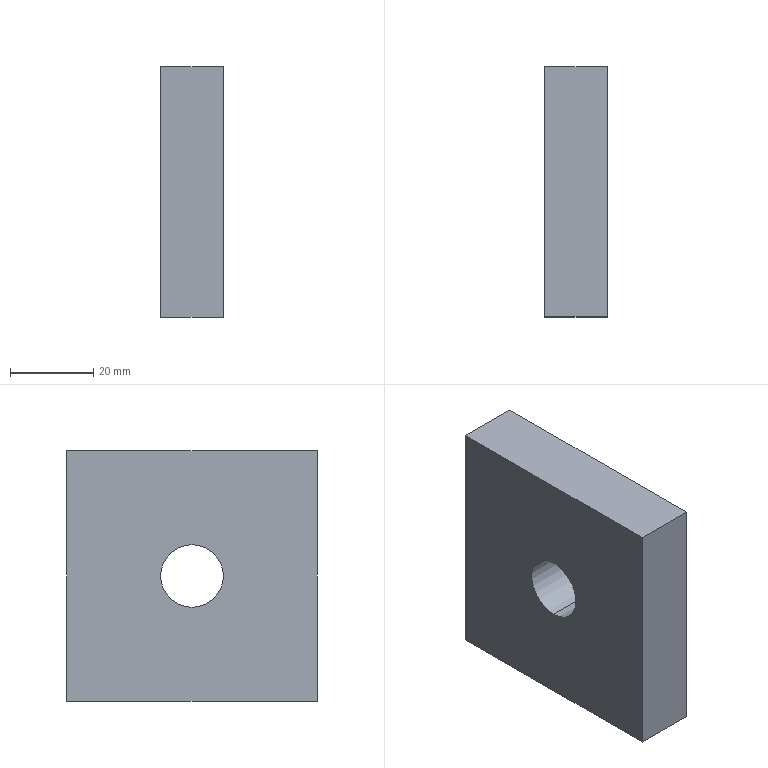Part | NX | 1 solid | 8 faces | box 15 x 60 x 60 mm | volume 51349 mm3 | plane 6 | cylinder 2 | commonest cylinder face diameters 15 x2
STEP:
#1=CARTESIAN_POINT('',(-250.326,-541.499,2402.586));
#2=VERTEX_POINT('',#1);
#3=CARTESIAN_POINT('',(-250.326,-541.499,2417.586));
#4=VERTEX_POINT('',#3);
#5=CARTESIAN_POINT('',(-250.326,-541.499,2410.086));
#6=DIRECTION('',(-1.,0.,0.));
#7=DIRECTION('',(0.,0.,1.));
#8=AXIS2_PLACEMENT_3D('',#5,#6,#7);
#9=CIRCLE('',#8,7.5);
#10=EDGE_CURVE('',#2,#4,#9,.T.);
#11=ORIENTED_EDGE('',*,*,#10,.T.);
#12=CARTESIAN_POINT('',(-235.326,-541.499,2417.586));
#13=VERTEX_POINT('',#12);
#14=CARTESIAN_POINT('',(-250.326,-541.499,2417.586));
#15=DIRECTION('',(1.,0.,0.));
#16=VECTOR('',#15,1.);
#17=LINE('',#14,#16);
#18=EDGE_CURVE('',#4,#13,#17,.T.);
#19=ORIENTED_EDGE('',*,*,#18,.T.);
#20=CARTESIAN_POINT('',(-235.326,-541.499,2402.586));
#21=VERTEX_POINT('',#20);
#22=CARTESIAN_POINT('',(-235.326,-541.499,2410.086));
#23=DIRECTION('',(-1.,0.,0.));
#24=DIRECTION('',(0.,0.,1.));
#25=AXIS2_PLACEMENT_3D('',#22,#23,#24);
#26=CIRCLE('',#25,7.5);
#27=EDGE_CURVE('',#21,#13,#26,.T.);
#28=ORIENTED_EDGE('',*,*,#27,.F.);
#29=CARTESIAN_POINT('',(-250.326,-541.499,2402.586));
#30=DIRECTION('',(-1.,0.,0.));
#31=VECTOR('',#30,1.);
#32=LINE('',#29,#31);
#33=EDGE_CURVE('',#21,#2,#32,.T.);
#34=ORIENTED_EDGE('',*,*,#33,.T.);
#35=EDGE_LOOP('',(#11,#19,#28,#34));
#36=FACE_OUTER_BOUND('',#35,.T.);
#37=CARTESIAN_POINT('',(-250.326,-541.499,2410.086));
#38=DIRECTION('',(1.,0.,0.));
#39=DIRECTION('',(0.,0.,-1.));
#40=AXIS2_PLACEMENT_3D('',#37,#38,#39);
#41=CYLINDRICAL_SURFACE('',#40,7.5);
#42=ADVANCED_FACE('',(#36),#41,.F.);
#43=CARTESIAN_POINT('',(-250.326,-511.499,2380.086));
#44=VERTEX_POINT('',#43);
#45=CARTESIAN_POINT('',(-250.326,-571.499,2380.086));
#46=VERTEX_POINT('',#45);
#47=CARTESIAN_POINT('',(-250.326,-511.499,2380.086));
#48=DIRECTION('',(0.,-1.,0.));
#49=VECTOR('',#48,1.);
#50=LINE('',#47,#49);
#51=EDGE_CURVE('',#44,#46,#50,.T.);
#52=ORIENTED_EDGE('',*,*,#51,.T.);
#53=CARTESIAN_POINT('',(-250.326,-571.499,2440.086));
#54=VERTEX_POINT('',#53);
#55=CARTESIAN_POINT('',(-250.326,-571.499,2380.086));
#56=DIRECTION('',(0.,0.,1.));
#57=VECTOR('',#56,1.);
#58=LINE('',#55,#57);
#59=EDGE_CURVE('',#46,#54,#58,.T.);
#60=ORIENTED_EDGE('',*,*,#59,.T.);
#61=CARTESIAN_POINT('',(-250.326,-511.499,2440.086));
#62=VERTEX_POINT('',#61);
#63=CARTESIAN_POINT('',(-250.326,-511.499,2440.086));
#64=DIRECTION('',(0.,1.,0.));
#65=VECTOR('',#64,1.);
#66=LINE('',#63,#65);
#67=EDGE_CURVE('',#54,#62,#66,.T.);
#68=ORIENTED_EDGE('',*,*,#67,.T.);
#69=CARTESIAN_POINT('',(-250.326,-511.499,2380.086));
#70=DIRECTION('',(0.,0.,-1.));
#71=VECTOR('',#70,1.);
#72=LINE('',#69,#71);
#73=EDGE_CURVE('',#62,#44,#72,.T.);
#74=ORIENTED_EDGE('',*,*,#73,.T.);
#75=EDGE_LOOP('',(#52,#60,#68,#74));
#76=FACE_BOUND('',#75,.T.);
#77=ORIENTED_EDGE('',*,*,#10,.F.);
#78=CARTESIAN_POINT('',(-250.326,-541.499,2410.086));
#79=DIRECTION('',(-1.,0.,0.));
#80=DIRECTION('',(0.,0.,1.));
#81=AXIS2_PLACEMENT_3D('',#78,#79,#80);
#82=CIRCLE('',#81,7.5);
#83=EDGE_CURVE('',#4,#2,#82,.T.);
#84=ORIENTED_EDGE('',*,*,#83,.F.);
#85=EDGE_LOOP('',(#77,#84));
#86=FACE_BOUND('',#85,.T.);
#87=CARTESIAN_POINT('',(-250.326,-571.499,2380.086));
#88=DIRECTION('',(-1.,0.,0.));
#89=DIRECTION('',(0.,0.,1.));
#90=AXIS2_PLACEMENT_3D('',#87,#88,#89);
#91=PLANE('',#90);
#92=ADVANCED_FACE('',(#76,#86),#91,.T.);
#93=CARTESIAN_POINT('',(-235.326,-511.499,2380.086));
#94=VERTEX_POINT('',#93);
#95=CARTESIAN_POINT('',(-235.326,-571.499,2380.086));
#96=VERTEX_POINT('',#95);
#97=CARTESIAN_POINT('',(-235.326,-511.499,2380.086));
#98=DIRECTION('',(0.,-1.,0.));
#99=VECTOR('',#98,1.);
#100=LINE('',#97,#99);
#101=EDGE_CURVE('',#94,#96,#100,.T.);
#102=ORIENTED_EDGE('',*,*,#101,.F.);
#103=CARTESIAN_POINT('',(-235.326,-511.499,2440.086));
#104=VERTEX_POINT('',#103);
#105=CARTESIAN_POINT('',(-235.326,-511.499,2380.086));
#106=DIRECTION('',(0.,0.,-1.));
#107=VECTOR('',#106,1.);
#108=LINE('',#105,#107);
#109=EDGE_CURVE('',#104,#94,#108,.T.);
#110=ORIENTED_EDGE('',*,*,#109,.F.);
#111=CARTESIAN_POINT('',(-235.326,-571.499,2440.086));
#112=VERTEX_POINT('',#111);
#113=CARTESIAN_POINT('',(-235.326,-511.499,2440.086));
#114=DIRECTION('',(0.,1.,0.));
#115=VECTOR('',#114,1.);
#116=LINE('',#113,#115);
#117=EDGE_CURVE('',#112,#104,#116,.T.);
#118=ORIENTED_EDGE('',*,*,#117,.F.);
#119=CARTESIAN_POINT('',(-235.326,-571.499,2380.086));
#120=DIRECTION('',(0.,0.,1.));
#121=VECTOR('',#120,1.);
#122=LINE('',#119,#121);
#123=EDGE_CURVE('',#96,#112,#122,.T.);
#124=ORIENTED_EDGE('',*,*,#123,.F.);
#125=EDGE_LOOP('',(#102,#110,#118,#124));
#126=FACE_BOUND('',#125,.T.);
#127=ORIENTED_EDGE('',*,*,#27,.T.);
#128=CARTESIAN_POINT('',(-235.326,-541.499,2410.086));
#129=DIRECTION('',(-1.,0.,0.));
#130=DIRECTION('',(0.,0.,1.));
#131=AXIS2_PLACEMENT_3D('',#128,#129,#130);
#132=CIRCLE('',#131,7.5);
#133=EDGE_CURVE('',#13,#21,#132,.T.);
#134=ORIENTED_EDGE('',*,*,#133,.T.);
#135=EDGE_LOOP('',(#127,#134));
#136=FACE_BOUND('',#135,.T.);
#137=CARTESIAN_POINT('',(-235.326,-571.499,2380.086));
#138=DIRECTION('',(-1.,0.,0.));
#139=DIRECTION('',(0.,0.,1.));
#140=AXIS2_PLACEMENT_3D('',#137,#138,#139);
#141=PLANE('',#140);
#142=ADVANCED_FACE('',(#126,#136),#141,.F.);
#143=ORIENTED_EDGE('',*,*,#101,.T.);
#144=CARTESIAN_POINT('',(-250.326,-571.499,2380.086));
#145=DIRECTION('',(1.,0.,0.));
#146=VECTOR('',#145,1.);
#147=LINE('',#144,#146);
#148=EDGE_CURVE('',#46,#96,#147,.T.);
#149=ORIENTED_EDGE('',*,*,#148,.F.);
#150=ORIENTED_EDGE('',*,*,#51,.F.);
#151=CARTESIAN_POINT('',(-250.326,-511.499,2380.086));
#152=DIRECTION('',(1.,0.,0.));
#153=VECTOR('',#152,1.);
#154=LINE('',#151,#153);
#155=EDGE_CURVE('',#44,#94,#154,.T.);
#156=ORIENTED_EDGE('',*,*,#155,.T.);
#157=EDGE_LOOP('',(#143,#149,#150,#156));
#158=FACE_OUTER_BOUND('',#157,.T.);
#159=CARTESIAN_POINT('',(-250.326,-511.499,2380.086));
#160=DIRECTION('',(0.,0.,1.));
#161=DIRECTION('',(0.,-1.,0.));
#162=AXIS2_PLACEMENT_3D('',#159,#160,#161);
#163=PLANE('',#162);
#164=ADVANCED_FACE('',(#158),#163,.F.);
#165=ORIENTED_EDGE('',*,*,#123,.T.);
#166=CARTESIAN_POINT('',(-250.326,-571.499,2440.086));
#167=DIRECTION('',(1.,0.,0.));
#168=VECTOR('',#167,1.);
#169=LINE('',#166,#168);
#170=EDGE_CURVE('',#54,#112,#169,.T.);
#171=ORIENTED_EDGE('',*,*,#170,.F.);
#172=ORIENTED_EDGE('',*,*,#59,.F.);
#173=ORIENTED_EDGE('',*,*,#148,.T.);
#174=EDGE_LOOP('',(#165,#171,#172,#173));
#175=FACE_OUTER_BOUND('',#174,.T.);
#176=CARTESIAN_POINT('',(-250.326,-571.499,2380.086));
#177=DIRECTION('',(0.,1.,0.));
#178=DIRECTION('',(0.,0.,1.));
#179=AXIS2_PLACEMENT_3D('',#176,#177,#178);
#180=PLANE('',#179);
#181=ADVANCED_FACE('',(#175),#180,.F.);
#182=ORIENTED_EDGE('',*,*,#117,.T.);
#183=CARTESIAN_POINT('',(-250.326,-511.499,2440.086));
#184=DIRECTION('',(1.,0.,0.));
#185=VECTOR('',#184,1.);
#186=LINE('',#183,#185);
#187=EDGE_CURVE('',#62,#104,#186,.T.);
#188=ORIENTED_EDGE('',*,*,#187,.F.);
#189=ORIENTED_EDGE('',*,*,#67,.F.);
#190=ORIENTED_EDGE('',*,*,#170,.T.);
#191=EDGE_LOOP('',(#182,#188,#189,#190));
#192=FACE_OUTER_BOUND('',#191,.T.);
#193=CARTESIAN_POINT('',(-250.326,-511.499,2440.086));
#194=DIRECTION('',(0.,0.,-1.));
#195=DIRECTION('',(0.,1.,0.));
#196=AXIS2_PLACEMENT_3D('',#193,#194,#195);
#197=PLANE('',#196);
#198=ADVANCED_FACE('',(#192),#197,.F.);
#199=ORIENTED_EDGE('',*,*,#109,.T.);
#200=ORIENTED_EDGE('',*,*,#155,.F.);
#201=ORIENTED_EDGE('',*,*,#73,.F.);
#202=ORIENTED_EDGE('',*,*,#187,.T.);
#203=EDGE_LOOP('',(#199,#200,#201,#202));
#204=FACE_OUTER_BOUND('',#203,.T.);
#205=CARTESIAN_POINT('',(-250.326,-511.499,2380.086));
#206=DIRECTION('',(0.,-1.,0.));
#207=DIRECTION('',(0.,0.,-1.));
#208=AXIS2_PLACEMENT_3D('',#205,#206,#207);
#209=PLANE('',#208);
#210=ADVANCED_FACE('',(#204),#209,.F.);
#211=ORIENTED_EDGE('',*,*,#18,.F.);
#212=ORIENTED_EDGE('',*,*,#83,.T.);
#213=ORIENTED_EDGE('',*,*,#33,.F.);
#214=ORIENTED_EDGE('',*,*,#133,.F.);
#215=EDGE_LOOP('',(#211,#212,#213,#214));
#216=FACE_OUTER_BOUND('',#215,.T.);
#217=CARTESIAN_POINT('',(-250.326,-541.499,2410.086));
#218=DIRECTION('',(1.,0.,0.));
#219=DIRECTION('',(0.,0.,-1.));
#220=AXIS2_PLACEMENT_3D('',#217,#218,#219);
#221=CYLINDRICAL_SURFACE('',#220,7.5);
#222=ADVANCED_FACE('',(#216),#221,.F.);
#223=CLOSED_SHELL('',(#42,#92,#142,#164,#181,#198,#210,#222));
#224=MANIFOLD_SOLID_BREP('',#223);
#225=(LENGTH_UNIT()NAMED_UNIT(*)SI_UNIT(.MILLI.,.METRE.));
#226=UNCERTAINTY_MEASURE_WITH_UNIT(LENGTH_MEASURE(0.00002),#225,'','');
#227=(NAMED_UNIT(*)PLANE_ANGLE_UNIT()SI_UNIT($,.RADIAN.));
#228=PLANE_ANGLE_MEASURE_WITH_UNIT(PLANE_ANGLE_MEASURE(0.01745),#227);
#229=DIMENSIONAL_EXPONENTS(0.,0.,0.,0.,0.,0.,0.);
#230=(CONVERSION_BASED_UNIT('DEGREE',#228)NAMED_UNIT(#229)PLANE_ANGLE_UNIT());
#231=(NAMED_UNIT(*)SI_UNIT($,.STERADIAN.)SOLID_ANGLE_UNIT());
#232=(GEOMETRIC_REPRESENTATION_CONTEXT(3)GLOBAL_UNCERTAINTY_ASSIGNED_CONTEXT((#226))GLOBAL_UNIT_ASSIGNED_CONTEXT((#225,#230,#231))REPRESENTATION_CONTEXT('',''));
#233=ADVANCED_BREP_SHAPE_REPRESENTATION('',(#224),#232);